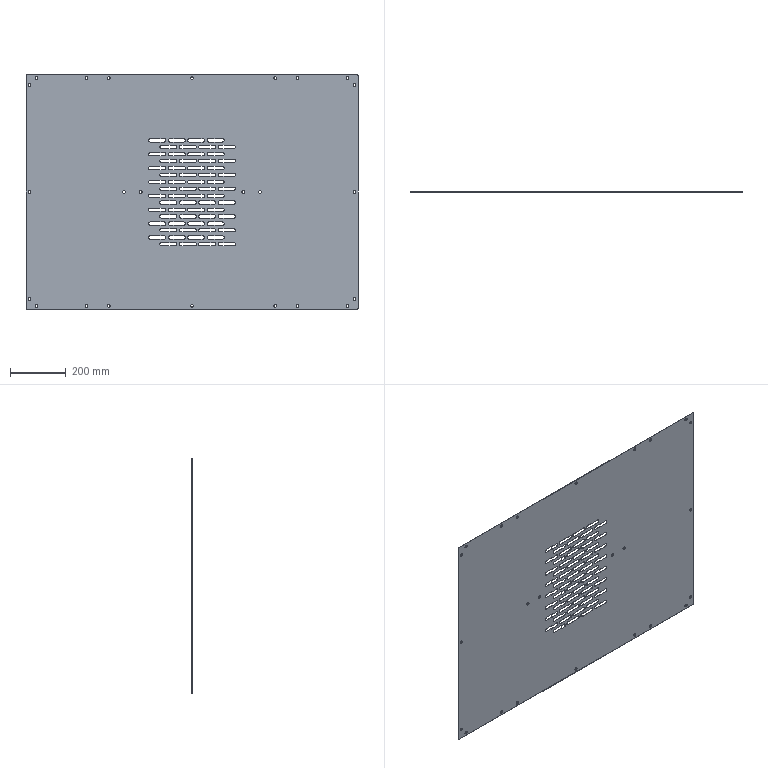Part | SolidWorks | features LPattern 4, HoleWzd 3, EdgeFlange 1, Fillet 1, FlatPattern 1, ICE 1, SMBaseFlange 1, SheetMetal 1 | 1 solid | 314 faces | box 1196 x 1.2 x 846 mm | volume 1157126 mm3 | cylinder 180 | plane 134 | commonest cylinder face diameters 12 x128 10 x52